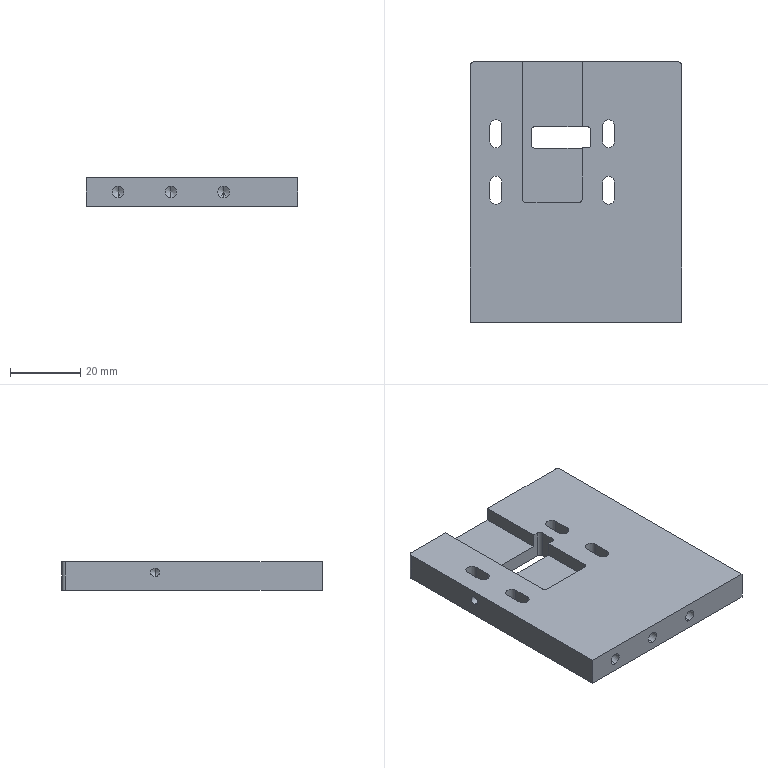Part | NX | features BREP 1 | 1 solid | 79 faces | box 60 x 74 x 8 mm | volume 30576 mm3 | plane 35 | cylinder 34 | cone 10 | commonest cylinder face diameters 2 x8 3.4 x8 7 x8 3.3 x6 2.5 x4